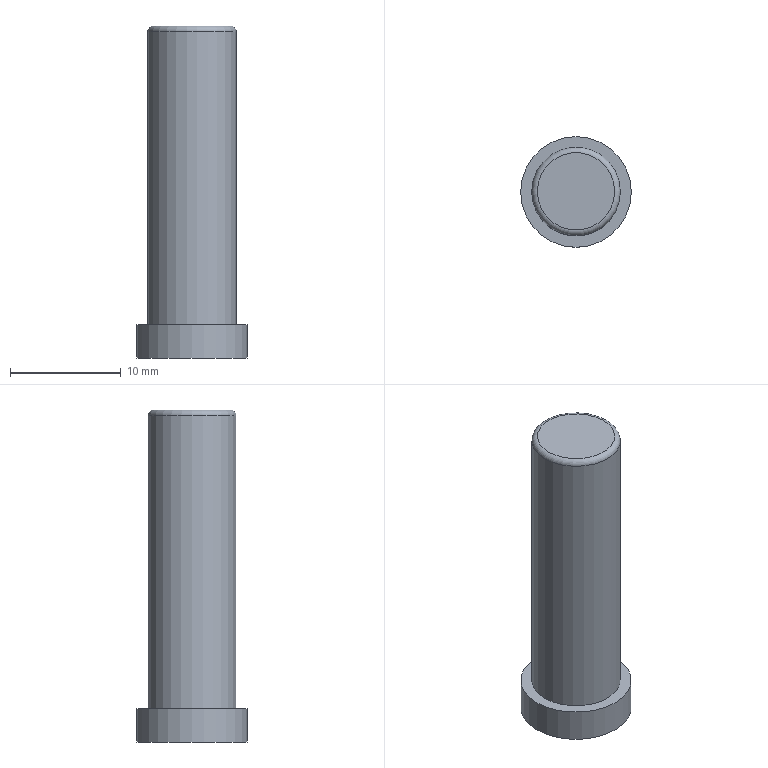Part | NX | features solid 2 | 1 solid | 6 faces | box 10 x 10 x 30 mm | volume 1591 mm3 | plane 3 | cylinder 2 | torus 1 | commonest cylinder face diameters 8 x1 10 x1
STEP:
#1=CARTESIAN_POINT('',(139.917,-35.784,1.5));
#2=VERTEX_POINT('',#1);
#3=CARTESIAN_POINT('',(136.417,-35.784,1.5));
#4=DIRECTION('',(0.,0.,-1.));
#5=DIRECTION('',(1.,0.,0.));
#6=AXIS2_PLACEMENT_3D('',#3,#4,#5);
#7=CIRCLE('',#6,3.5);
#8=EDGE_CURVE('',#2,#2,#7,.T.);
#9=ORIENTED_EDGE('',*,*,#8,.F.);
#10=EDGE_LOOP('',(#9));
#11=FACE_BOUND('',#10,.T.);
#12=CARTESIAN_POINT('',(136.417,-35.784,1.5));
#13=DIRECTION('',(0.,0.,1.));
#14=DIRECTION('',(-1.,0.,0.));
#15=AXIS2_PLACEMENT_3D('',#12,#13,#14);
#16=PLANE('',#15);
#17=ADVANCED_FACE('',(#11),#16,.T.);
#18=CARTESIAN_POINT('',(140.417,-35.784,-25.5));
#19=VERTEX_POINT('',#18);
#20=CARTESIAN_POINT('',(136.417,-35.784,-25.5));
#21=DIRECTION('',(0.,0.,1.));
#22=DIRECTION('',(1.,0.,0.));
#23=AXIS2_PLACEMENT_3D('',#20,#21,#22);
#24=CIRCLE('',#23,4.);
#25=EDGE_CURVE('',#19,#19,#24,.T.);
#26=ORIENTED_EDGE('',*,*,#25,.T.);
#27=EDGE_LOOP('',(#26));
#28=FACE_BOUND('',#27,.T.);
#29=CARTESIAN_POINT('',(140.417,-35.784,1.));
#30=VERTEX_POINT('',#29);
#31=CARTESIAN_POINT('',(136.417,-35.784,1.));
#32=DIRECTION('',(0.,0.,1.));
#33=DIRECTION('',(1.,0.,0.));
#34=AXIS2_PLACEMENT_3D('',#31,#32,#33);
#35=CIRCLE('',#34,4.);
#36=EDGE_CURVE('',#30,#30,#35,.T.);
#37=ORIENTED_EDGE('',*,*,#36,.F.);
#38=EDGE_LOOP('',(#37));
#39=FACE_BOUND('',#38,.T.);
#40=CARTESIAN_POINT('',(136.417,-35.784,-41.5));
#41=DIRECTION('',(0.,0.,1.));
#42=DIRECTION('',(-1.,0.,0.));
#43=AXIS2_PLACEMENT_3D('',#40,#41,#42);
#44=CYLINDRICAL_SURFACE('',#43,4.);
#45=ADVANCED_FACE('',(#28,#39),#44,.T.);
#46=ORIENTED_EDGE('',*,*,#8,.T.);
#47=EDGE_LOOP('',(#46));
#48=FACE_BOUND('',#47,.T.);
#49=ORIENTED_EDGE('',*,*,#36,.T.);
#50=EDGE_LOOP('',(#49));
#51=FACE_BOUND('',#50,.T.);
#52=CARTESIAN_POINT('',(136.417,-35.784,1.));
#53=DIRECTION('',(0.,0.,1.));
#54=DIRECTION('',(-1.,0.,0.));
#55=AXIS2_PLACEMENT_3D('',#52,#53,#54);
#56=TOROIDAL_SURFACE('',#55,3.5,0.5);
#57=ADVANCED_FACE('',(#48,#51),#56,.T.);
#58=ORIENTED_EDGE('',*,*,#25,.F.);
#59=EDGE_LOOP('',(#58));
#60=FACE_BOUND('',#59,.T.);
#61=CARTESIAN_POINT('',(141.417,-35.784,-25.5));
#62=VERTEX_POINT('',#61);
#63=CARTESIAN_POINT('',(136.417,-35.784,-25.5));
#64=DIRECTION('',(0.,0.,1.));
#65=DIRECTION('',(1.,0.,0.));
#66=AXIS2_PLACEMENT_3D('',#63,#64,#65);
#67=CIRCLE('',#66,5.);
#68=EDGE_CURVE('',#62,#62,#67,.T.);
#69=ORIENTED_EDGE('',*,*,#68,.T.);
#70=EDGE_LOOP('',(#69));
#71=FACE_BOUND('',#70,.T.);
#72=CARTESIAN_POINT('',(136.417,-35.784,-25.5));
#73=DIRECTION('',(0.,0.,1.));
#74=DIRECTION('',(-1.,0.,0.));
#75=AXIS2_PLACEMENT_3D('',#72,#73,#74);
#76=PLANE('',#75);
#77=ADVANCED_FACE('',(#60,#71),#76,.T.);
#78=ORIENTED_EDGE('',*,*,#68,.F.);
#79=EDGE_LOOP('',(#78));
#80=FACE_BOUND('',#79,.T.);
#81=CARTESIAN_POINT('',(141.417,-35.784,-28.5));
#82=VERTEX_POINT('',#81);
#83=CARTESIAN_POINT('',(136.417,-35.784,-28.5));
#84=DIRECTION('',(0.,0.,-1.));
#85=DIRECTION('',(1.,0.,0.));
#86=AXIS2_PLACEMENT_3D('',#83,#84,#85);
#87=CIRCLE('',#86,5.);
#88=EDGE_CURVE('',#82,#82,#87,.T.);
#89=ORIENTED_EDGE('',*,*,#88,.F.);
#90=EDGE_LOOP('',(#89));
#91=FACE_BOUND('',#90,.T.);
#92=CARTESIAN_POINT('',(136.417,-35.784,-28.5));
#93=DIRECTION('',(0.,0.,1.));
#94=DIRECTION('',(-1.,0.,0.));
#95=AXIS2_PLACEMENT_3D('',#92,#93,#94);
#96=CYLINDRICAL_SURFACE('',#95,5.);
#97=ADVANCED_FACE('',(#80,#91),#96,.T.);
#98=ORIENTED_EDGE('',*,*,#88,.T.);
#99=EDGE_LOOP('',(#98));
#100=FACE_BOUND('',#99,.T.);
#101=CARTESIAN_POINT('',(136.417,-35.784,-28.5));
#102=DIRECTION('',(0.,0.,-1.));
#103=DIRECTION('',(1.,0.,0.));
#104=AXIS2_PLACEMENT_3D('',#101,#102,#103);
#105=PLANE('',#104);
#106=ADVANCED_FACE('',(#100),#105,.T.);
#107=CLOSED_SHELL('',(#17,#45,#57,#77,#97,#106));
#108=MANIFOLD_SOLID_BREP('',#107);
#109=(LENGTH_UNIT()NAMED_UNIT(*)SI_UNIT(.MILLI.,.METRE.));
#110=UNCERTAINTY_MEASURE_WITH_UNIT(LENGTH_MEASURE(0.00001),#109,'','');
#111=(NAMED_UNIT(*)PLANE_ANGLE_UNIT()SI_UNIT($,.RADIAN.));
#112=(NAMED_UNIT(*)SI_UNIT($,.STERADIAN.)SOLID_ANGLE_UNIT());
#113=(GEOMETRIC_REPRESENTATION_CONTEXT(3)GLOBAL_UNCERTAINTY_ASSIGNED_CONTEXT((#110))GLOBAL_UNIT_ASSIGNED_CONTEXT((#109,#111,#112))REPRESENTATION_CONTEXT('',''));
#114=ADVANCED_BREP_SHAPE_REPRESENTATION('',(#108),#113);